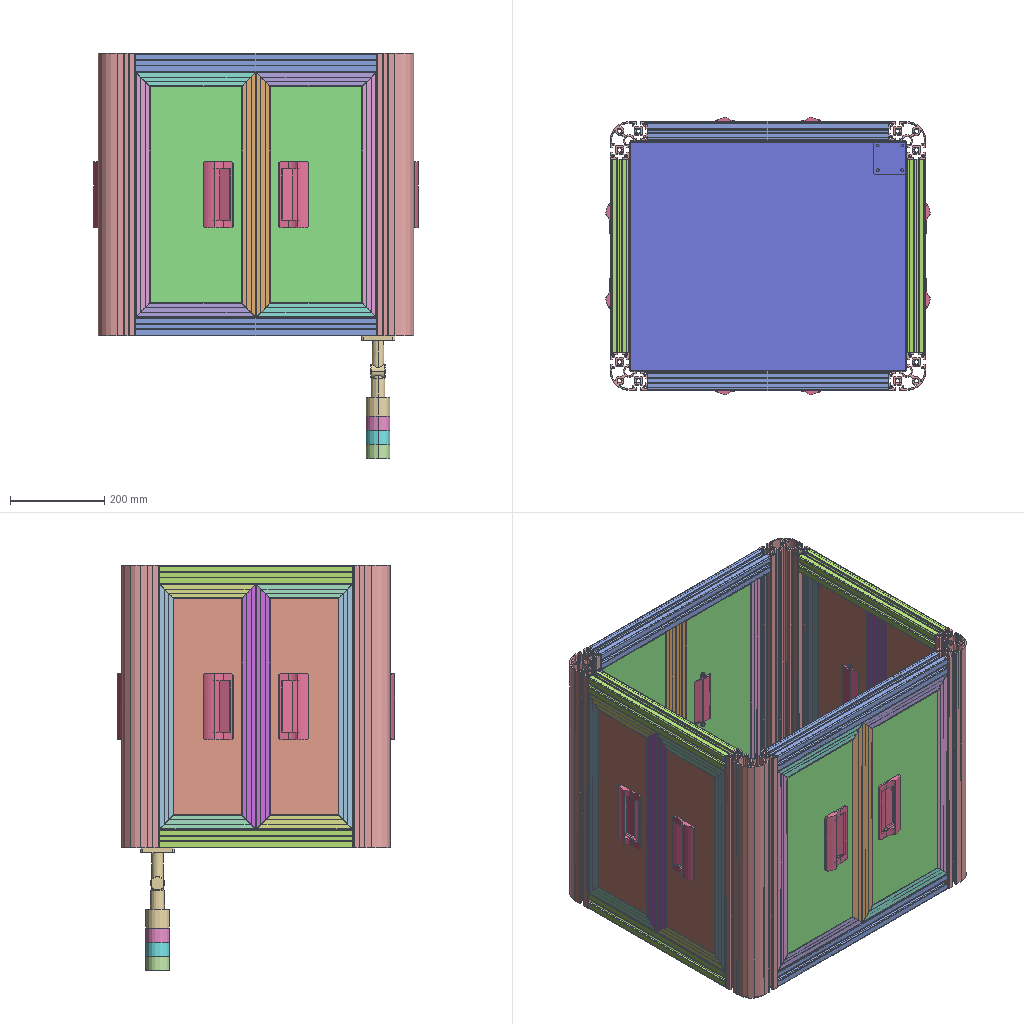Assembly | SolidWorks | 26 different items | 56 placed | box 688 x 588 x 861 mm
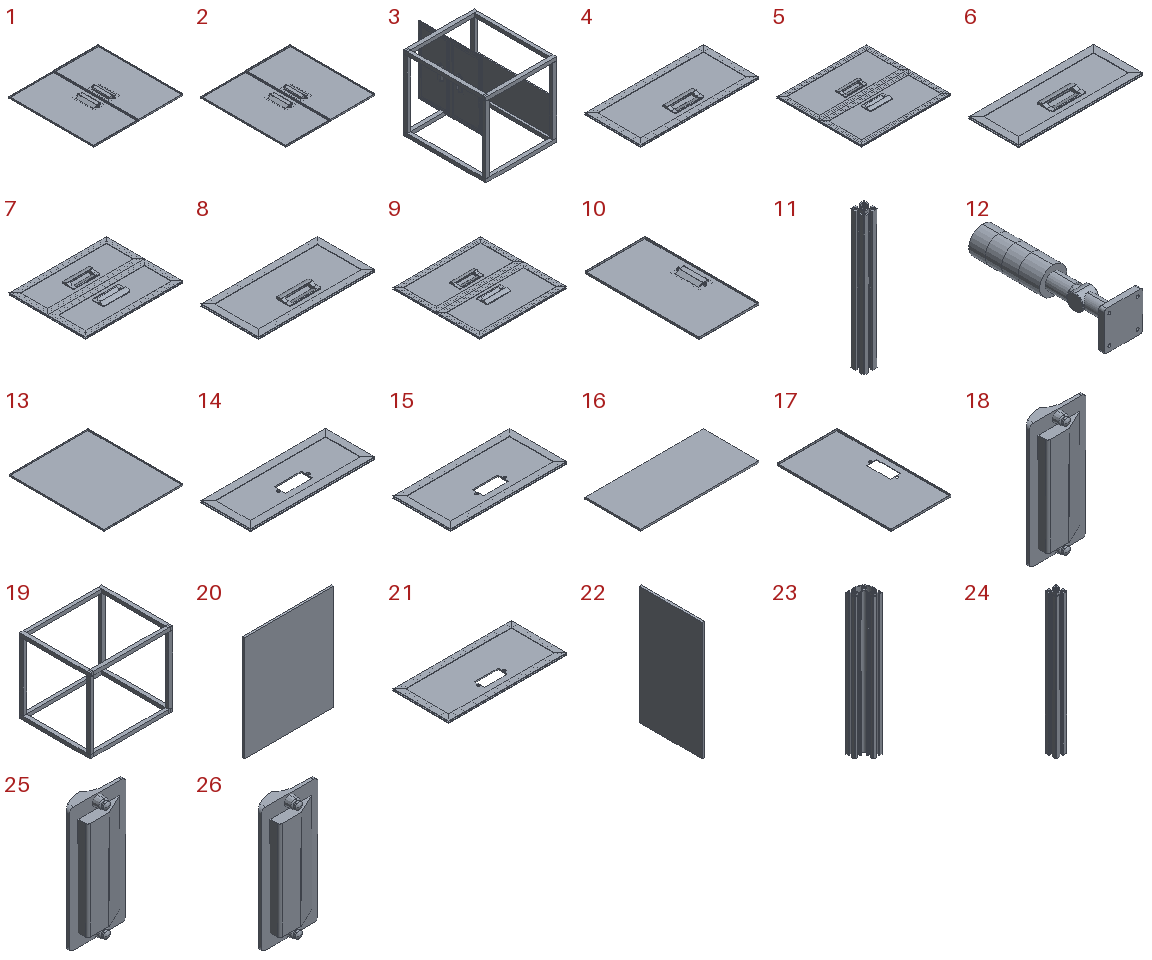Parts list (item | name | quantity | parent item | size | volume | features):
1 | (subassembly) | x1 | - | 570 x 540 x 23.592 mm | 738190 mm3 | -
2 | (subassembly) | x1 | - | 570 x 540 x 23.592 mm | 738190 mm3 | -
3 | (subassembly) | x1 | - | 600 x 890.825 x 630 mm | 10208073 mm3 | -
4 | (subassembly) | x1 | - | 570 x 270 x 23.592 mm | 859037 mm3 | -
5 | (subassembly) | x1 | - | 570 x 540 x 23.592 mm | 1718073 mm3 | -
6 | (subassembly) | x4 | in 7 | 520 x 205 x 23.592 mm | 599609 mm3 | -
7 | (subassembly) | x2 | - | 520 x 410 x 23.592 mm | 1199217 mm3 | -
8 | (subassembly) | x4 | in 9 | 520 x 255 x 23.592 mm | 742295 mm3 | -
9 | (subassembly) | x2 | - | 520 x 510 x 23.592 mm | 1484589 mm3 | -
10 | (subassembly) | x1 | - | 285 x 540 x 23.592 mm | 369095 mm3 | -
11 | - | x4 | - | 40 x 40 x 410 mm | 287601 mm3 | features Extrusion 1
12 | - | x1 | - | 72 x 260.521 x 72 mm | 382291 mm3 | features BaseBody 4
13 | - | x1 | - | 490 x 590 x 10 mm | 609167 mm3 | features EdgeFlange 1, FlatPattern 1, SMBaseFlange 1, SheetMetal 1
14 | - | x4 | in 6 | 520 x 205 x 10 mm | 550676 mm3 | features ICE 2, WeldMemberFeat 1, WeldmentFeature 1
15 | - | x4 | in 8 | 520 x 255 x 10 mm | 693362 mm3 | features ICE 2, WeldMemberFeat 1, WeldmentFeature 1
16 | - | x1 | - | 640 x 300 x 10 mm | 1920000 mm3 | features Extrusion 1
17 | - | x1 | - | 285 x 540 x 10 mm | 320162 mm3 | features EdgeFlange 1, FlatPattern 1, ICE 1, SMBaseFlange 1, SheetMetal 1
18 | - | x1 | - | 64 x 23.592 x 140 mm | 48933 mm3 | features BaseBody 1
19 | - | x1 | - | 700 x 600 x 630 mm | 6570000 mm3 | features WeldMemberFeat 2, 3DProfileFeature 1, WeldCornerFeat 1, WeldmentFeature 1
20 | - | x1 | - | 463.2 x 10.2 x 543.2 mm | 2566424 mm3 | features Extrusion 1
21 | - | x1 | - | 570 x 270 x 10 mm | 810104 mm3 | features ICE 2, WeldMemberFeat 1, WeldmentFeature 1
22 | - | x1 | - | 10.5 x 300 x 563.2 mm | 1774080 mm3 | features Extrusion 1
23 | - | x4 | - | 80 x 80 x 600 mm | 1006193 mm3 | features Extrusion 1
24 | - | x4 | - | 40 x 40 x 510 mm | 357748 mm3 | features Extrusion 1
25 | - | x8 | in 6, 8 | 64 x 23.592 x 140 mm | 48933 mm3 | features BaseBody 1
26 | - | x1 | - | 64 x 23.592 x 140 mm | 48933 mm3 | features BaseBody 1
Mates (type | each side: item.copy, entity, surface, feature):
In the top assembly
Coincident | 23.1 face plane Boss-Extrude1 | 24.1 face plane Boss-Extrude1 | 3 times
Coincident | 23.1 face plane Boss-Extrude1 | 23.2 face plane Boss-Extrude1
Coincident | 24.1 face plane Boss-Extrude1 | 23.2 face plane Boss-Extrude1 | 2 times
Coincident | 23.2 face plane Boss-Extrude1 | 11.1 face plane Boss-Extrude1 | 3 times
Coincident | 11.1 face plane Boss-Extrude1 | 23.3 face plane Boss-Extrude1 | 3 times
Coincident | 23.3 face plane Boss-Extrude1 | 24.2 face plane Boss-Extrude1 | 2 times
Coincident | 11.1 face plane Boss-Extrude1 | 24.2 face plane Boss-Extrude1
Coincident | 24.2 face plane Boss-Extrude1 | 23.4 face plane Boss-Extrude1 | 3 times
Coincident | 23.4 face plane Boss-Extrude1 | 11.2 face plane Boss-Extrude1 | 3 times
Coincident | 23.3 face plane Boss-Extrude1 | 24.3 face plane Boss-Extrude1 | 3 times
Coincident | 23.3 face plane Boss-Extrude1 | 11.3 face plane Boss-Extrude1 | 3 times
Coincident | 23.2 face plane Boss-Extrude1 | 24.4 face plane Boss-Extrude1
Coincident | 11.3 face plane Boss-Extrude1 | 24.4 face plane Boss-Extrude1
Coincident | 23.1 face plane Boss-Extrude1 | 24.4 face plane Boss-Extrude1
Coincident | 23.1 face plane Boss-Extrude1 | 11.4 face plane Boss-Extrude1 | 3 times
Coincident | 24.1 face plane Boss-Extrude1 | 9.1 plane
Coincident | 24.4 face plane Boss-Extrude1 | 9.1 plane
Coincident | 23.2 face plane Boss-Extrude1 | 9.1 plane
Coincident | 11.1 face plane Boss-Extrude1 | 7.1 plane
Coincident | 11.3 face plane Boss-Extrude1 | 7.1 plane
Coincident | 23.3 face plane Boss-Extrude1 | 7.1 plane
Coincident | 24.3 face plane Boss-Extrude1 | 15.1 face plane Aluminium profile 20 X 20 X 2(1) | 2 times
Coincident | 23.4 face plane Boss-Extrude1 | 15.1 face plane Aluminium profile 20 X 20 X 2(1)
Coincident | 24.3 face plane Boss-Extrude1 | 13.1 plane
Coincident | 24.4 face plane Boss-Extrude1 | 13.1 plane
Coincident | 11.4 face plane Boss-Extrude1 | 13.1 plane
Coincident | 11.4 face plane Boss-Extrude1 | 14.1 face plane Aluminium profile 20 X 20 X 2(1) | 2 times
Coincident | 23.4 face plane Boss-Extrude1 | 14.2 face plane Aluminium profile 20 X 20 X 2(1)
Coincident | 13.1 face plane Base-Flange1 | 12.1 face plane Input 12
Coincident | 23.1 face plane Boss-Extrude1 | 12.1 face plane Input 12 | 2 times
In subassembly 7
Coincident | 14.3 face plane Boss-Extrude1 | 14.4 face plane Boss-Extrude1
Coincident | 14.3 face plane Aluminium profile 20 X 20 X 2(1) | 14.4 face plane Aluminium profile 20 X 20 X 2(1) | 2 times
In subassembly 6
Coincident | 14.5 face plane Boss-Extrude1 | 25.1 face plane Input 1
Concentric | 14.5 face cylinder Cut-Extrude1 | 25.1 face cone Input 1 | 2 times
In subassembly 9
Coincident | 15.2 face plane Boss-Extrude1 | 15.3 face plane Boss-Extrude1
Coincident | 15.2 face plane Aluminium profile 20 X 20 X 2(1) | 15.3 face plane Aluminium profile 20 X 20 X 2(1) | 2 times
In subassembly 8
Coincident | 15.4 face plane Boss-Extrude1 | 25.1 face plane Input 1
Concentric | 15.4 face cylinder Cut-Extrude1 | 25.1 face cone Input 1 | 2 times